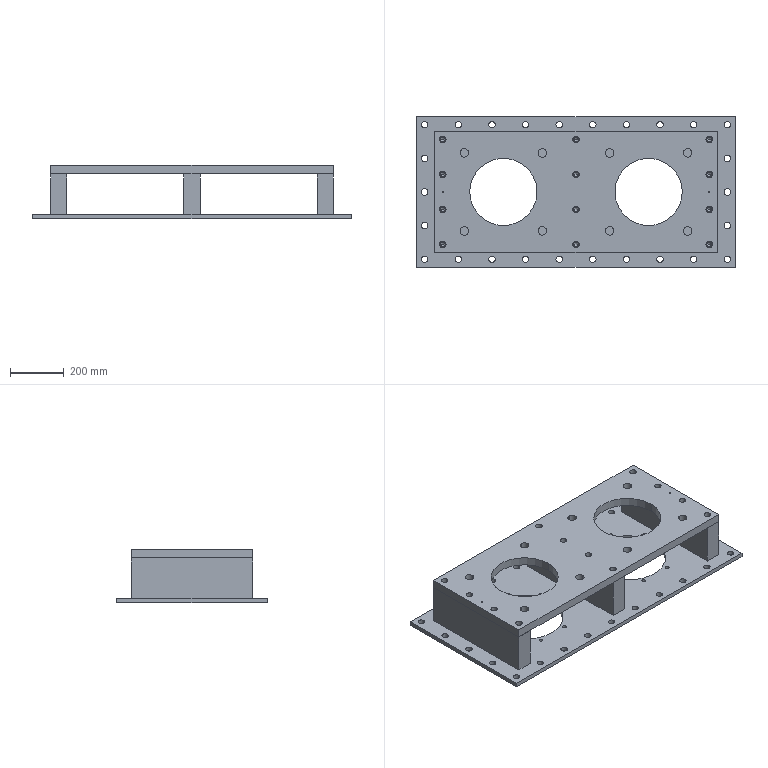Part | SolidWorks | features AEMSimFeature 1 | 5 solids | 214 faces | box 1185 x 560 x 198 mm | volume 31946209 mm3 | cylinder 160 | plane 30 | cone 24 | commonest cylinder face diameters 24 x76 14 x32 17.5 x24 32 x16 6 x4 250 x4